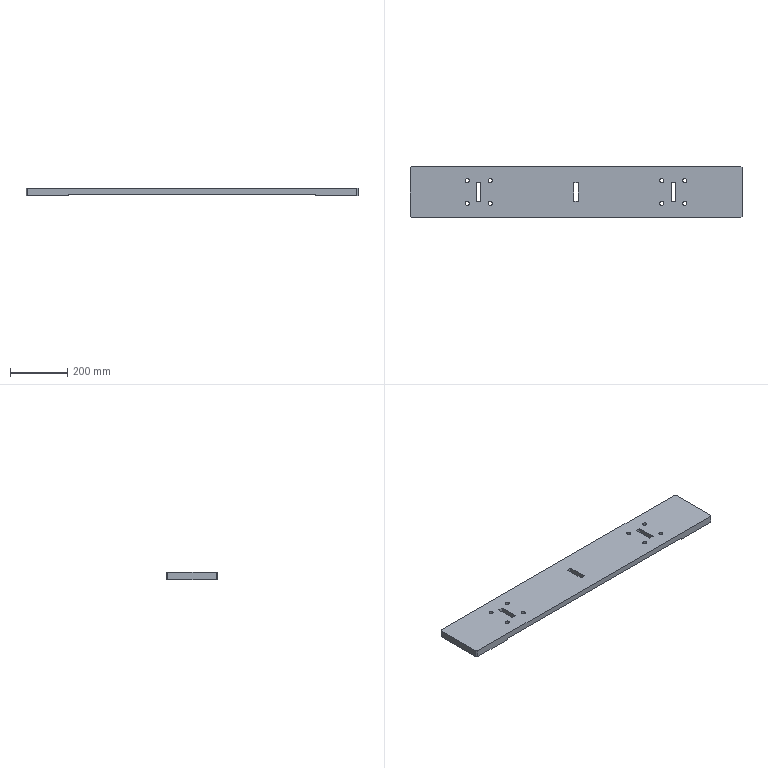Part | SolidWorks | features BaseBody 1 | 1 solid | 58 faces | box 1160 x 180 x 25 mm | volume 4356566 mm3 | plane 26 | cone 16 | cylinder 16 | commonest cylinder face diameters 14 x16